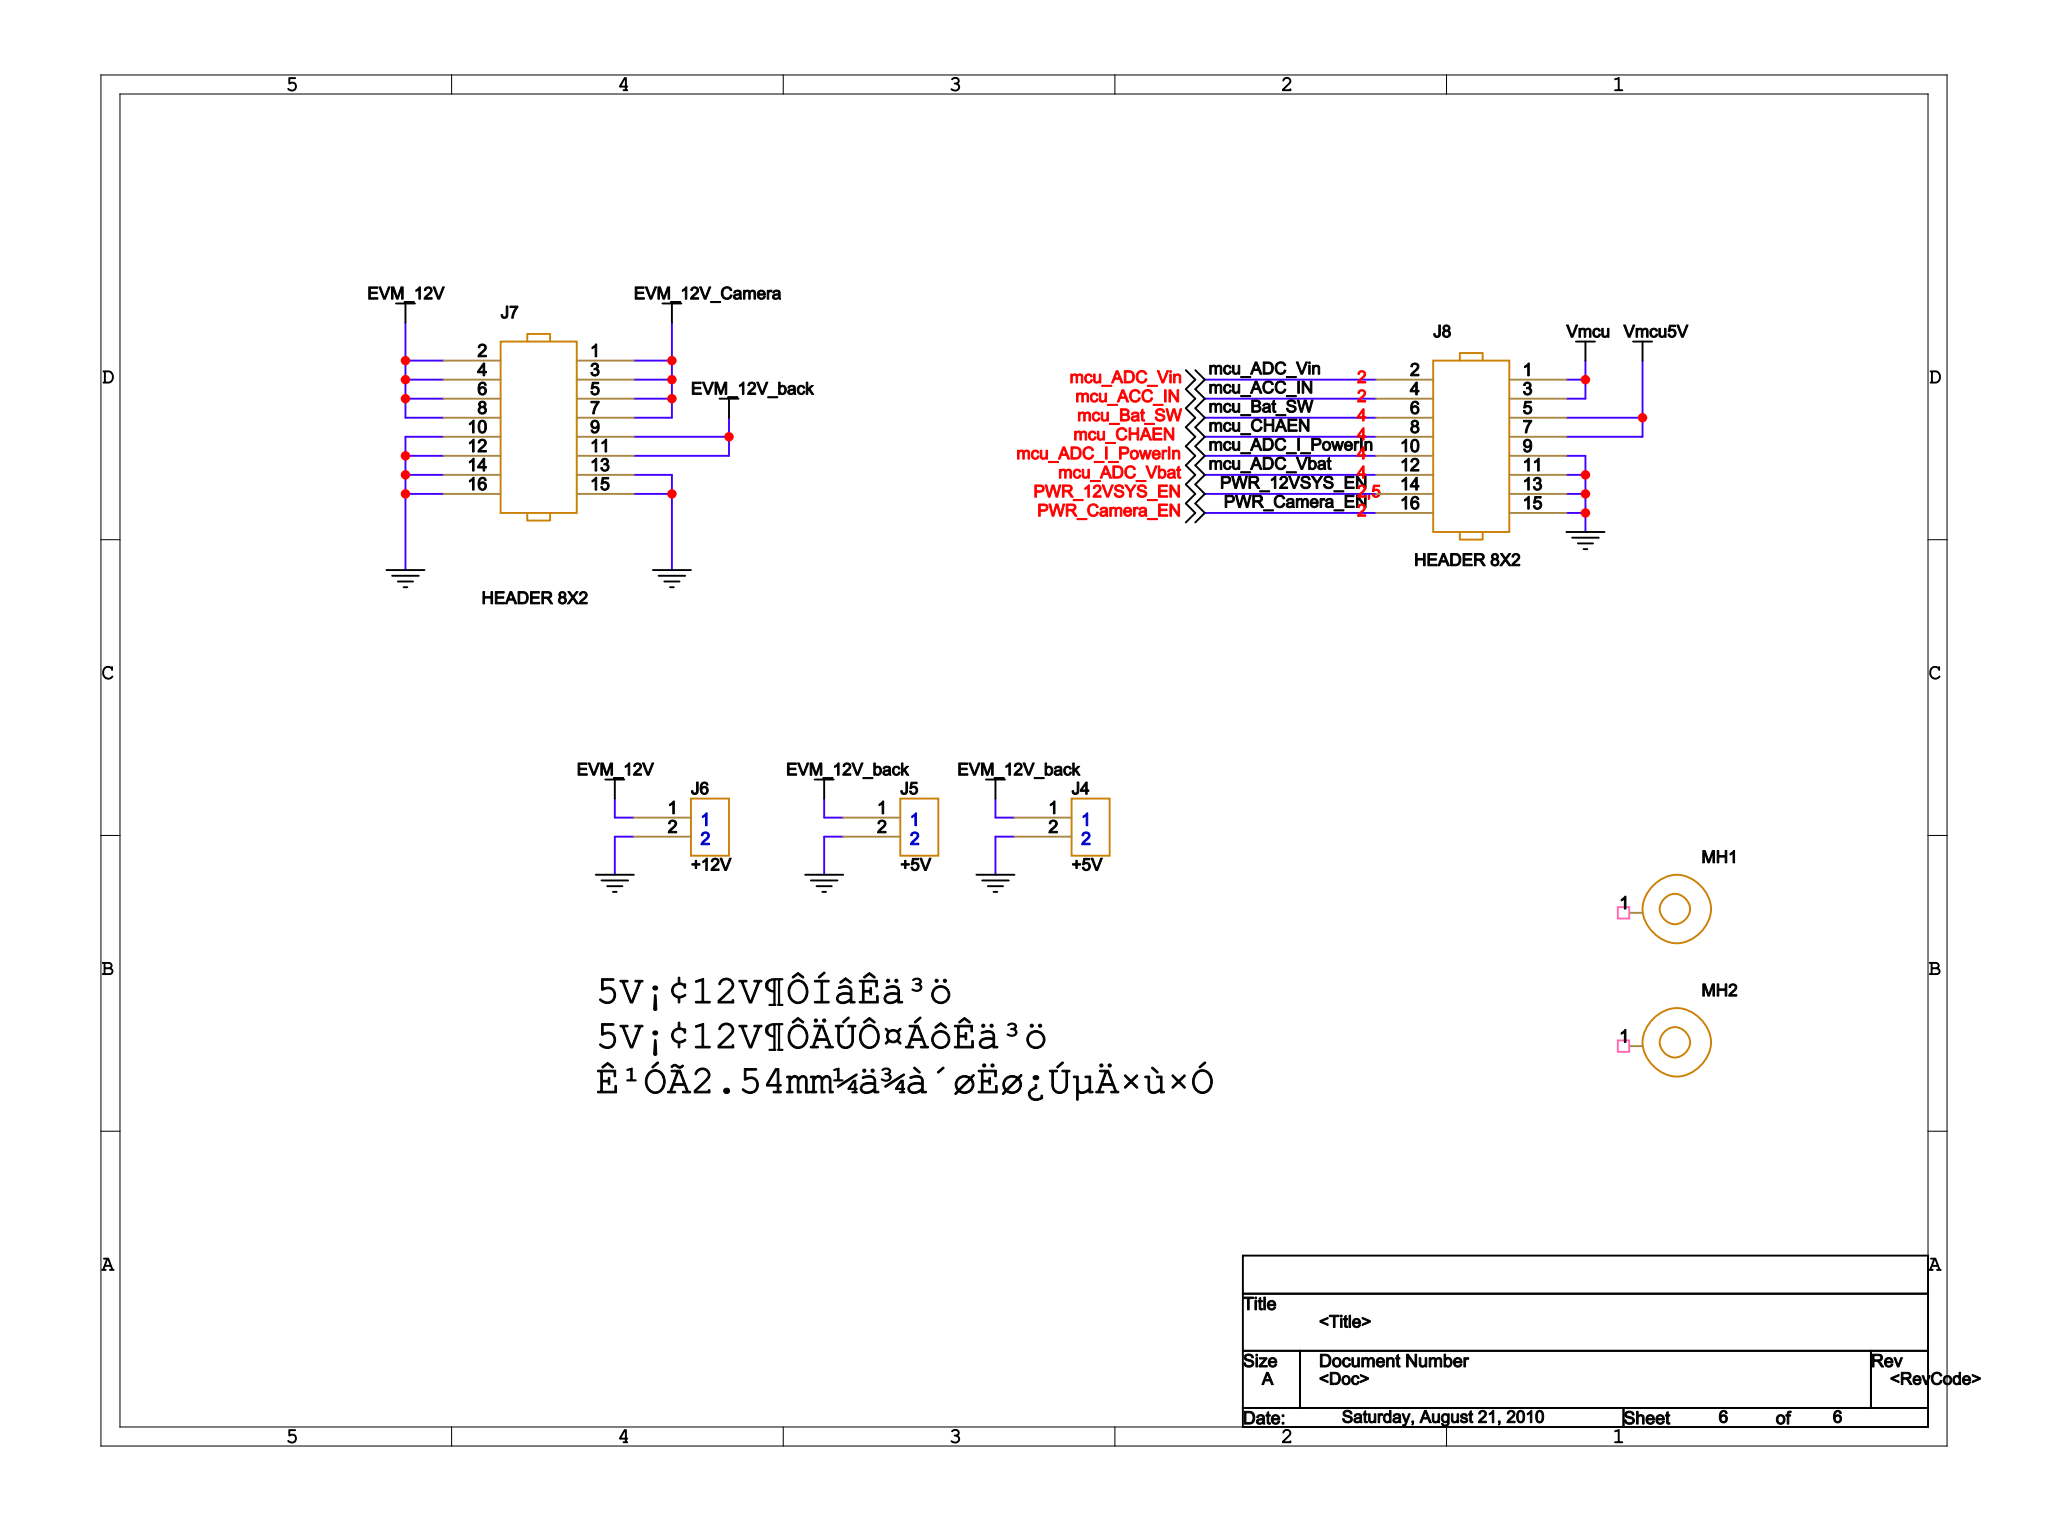Circuit board | Cadence Allegro | 241 parts | 116 nets | one sheet of the schematic
Parts on this sheet (reference | value | footprint):
J5 | +5V | HDR2MM54_1X2
J6 | +12V | HDR2MM54_1X2
J7 | HEADER 8X2 | HDR2MM54_2X8
J8 | HEADER 8X2 | HDR2MM54_2X8
Nets of these parts (net: part-pin ...):
GND: J5-2 J6-2 J7-10 J7-12 J7-13 J7-14 J7-15 J7-16 J8-9 J8-11 J8-13 J8-15
MCU_ADC_VIN: J8-2
EVM_12V_CAMERA: J7-1 J7-3 J7-5 J7-7
VMCU5V: J8-5 J8-7
VMCU: J8-1 J8-3
EVM_12V: J6-1 J7-2 J7-4 J7-6 J7-8
EVM_12V_BACK: J5-1 J7-9 J7-11
MCU_ADC_I_POWERIN: J8-10
PWR_CAMERA_EN: J8-16
PWR_12VSYS_EN: J8-14
MCU_ACC_IN: J8-4
MCU_ADC_VBAT: J8-12
MCU_CHAEN: J8-8
MCU_BAT_SW: J8-6